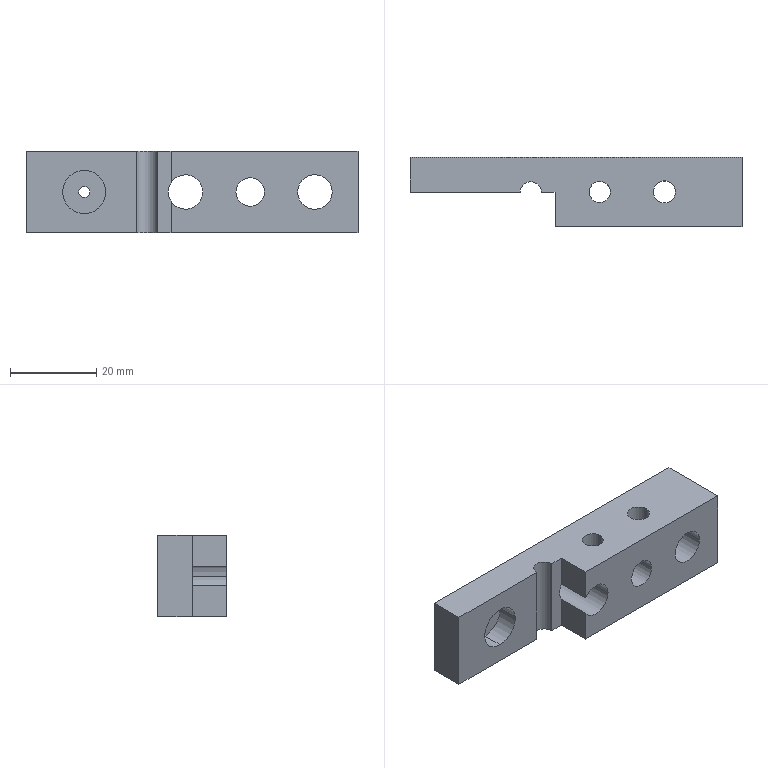Part | SolidWorks | features ICE 2, Extrusion 1 | 1 solid | 26 faces | box 77 x 16 x 19 mm | volume 14859 mm3 | cylinder 15 | plane 11 | commonest cylinder face diameters 8 x4 4.917 x3 2.599 x2 5.153 x2 6.647 x2 10 x2
STEP:
#1=CARTESIAN_POINT('',(13.5,5.,14.5));
#2=VERTEX_POINT('',#1);
#3=CARTESIAN_POINT('',(13.5,5.,4.5));
#4=VERTEX_POINT('',#3);
#5=CARTESIAN_POINT('',(13.5,5.,9.5));
#6=DIRECTION('',(0.,-1.,0.));
#7=DIRECTION('',(0.,0.,-1.));
#8=AXIS2_PLACEMENT_3D('',#5,#6,#7);
#9=CIRCLE('',#8,5.);
#10=EDGE_CURVE('',#2,#4,#9,.T.);
#11=ORIENTED_EDGE('',*,*,#10,.F.);
#12=CARTESIAN_POINT('',(13.5,0.,14.5));
#13=VERTEX_POINT('',#12);
#14=CARTESIAN_POINT('',(13.5,5.,14.5));
#15=DIRECTION('',(0.,-1.,0.));
#16=VECTOR('',#15,1000.);
#17=LINE('',#14,#16);
#18=EDGE_CURVE('',#2,#13,#17,.T.);
#19=ORIENTED_EDGE('',*,*,#18,.T.);
#20=CARTESIAN_POINT('',(13.5,0.,4.5));
#21=VERTEX_POINT('',#20);
#22=CARTESIAN_POINT('',(13.5,0.,9.5));
#23=DIRECTION('',(0.,-1.,0.));
#24=DIRECTION('',(0.,0.,-1.));
#25=AXIS2_PLACEMENT_3D('',#22,#23,#24);
#26=CIRCLE('',#25,5.);
#27=EDGE_CURVE('',#13,#21,#26,.T.);
#28=ORIENTED_EDGE('',*,*,#27,.T.);
#29=CARTESIAN_POINT('',(13.5,5.,4.5));
#30=DIRECTION('',(0.,-1.,0.));
#31=VECTOR('',#30,1000.);
#32=LINE('',#29,#31);
#33=EDGE_CURVE('',#4,#21,#32,.T.);
#34=ORIENTED_EDGE('',*,*,#33,.F.);
#35=EDGE_LOOP('',(#11,#19,#28,#34));
#36=FACE_OUTER_BOUND('',#35,.T.);
#37=CARTESIAN_POINT('',(13.5,5.,9.5));
#38=DIRECTION('',(0.,-1.,0.));
#39=DIRECTION('',(0.,0.,-1.));
#40=AXIS2_PLACEMENT_3D('',#37,#38,#39);
#41=CYLINDRICAL_SURFACE('',#40,5.);
#42=ADVANCED_FACE('',(#36),#41,.F.);
#43=CARTESIAN_POINT('',(71.,-7.907,9.5));
#44=VERTEX_POINT('',#43);
#45=CARTESIAN_POINT('',(63.,-7.907,9.5));
#46=VERTEX_POINT('',#45);
#47=CARTESIAN_POINT('',(67.,-7.907,9.5));
#48=DIRECTION('',(0.,1.,0.));
#49=DIRECTION('',(-1.,0.,0.));
#50=AXIS2_PLACEMENT_3D('',#47,#48,#49);
#51=CIRCLE('',#50,4.);
#52=EDGE_CURVE('',#44,#46,#51,.T.);
#53=ORIENTED_EDGE('',*,*,#52,.F.);
#54=CARTESIAN_POINT('',(71.,8.093,9.5));
#55=VERTEX_POINT('',#54);
#56=CARTESIAN_POINT('',(71.,-7.907,9.5));
#57=DIRECTION('',(0.,1.,0.));
#58=VECTOR('',#57,1000.);
#59=LINE('',#56,#58);
#60=EDGE_CURVE('',#44,#55,#59,.T.);
#61=ORIENTED_EDGE('',*,*,#60,.T.);
#62=CARTESIAN_POINT('',(63.,8.093,9.5));
#63=VERTEX_POINT('',#62);
#64=CARTESIAN_POINT('',(67.,8.093,9.5));
#65=DIRECTION('',(0.,1.,0.));
#66=DIRECTION('',(-1.,0.,0.));
#67=AXIS2_PLACEMENT_3D('',#64,#65,#66);
#68=CIRCLE('',#67,4.);
#69=EDGE_CURVE('',#55,#63,#68,.T.);
#70=ORIENTED_EDGE('',*,*,#69,.T.);
#71=CARTESIAN_POINT('',(63.,-7.907,9.5));
#72=DIRECTION('',(0.,1.,0.));
#73=VECTOR('',#72,1000.);
#74=LINE('',#71,#73);
#75=EDGE_CURVE('',#46,#63,#74,.T.);
#76=ORIENTED_EDGE('',*,*,#75,.F.);
#77=EDGE_LOOP('',(#53,#61,#70,#76));
#78=FACE_OUTER_BOUND('',#77,.T.);
#79=CARTESIAN_POINT('',(67.,-7.907,9.5));
#80=DIRECTION('',(0.,1.,0.));
#81=DIRECTION('',(-1.,0.,0.));
#82=AXIS2_PLACEMENT_3D('',#79,#80,#81);
#83=CYLINDRICAL_SURFACE('',#82,4.);
#84=ADVANCED_FACE('',(#78),#83,.F.);
#85=CARTESIAN_POINT('',(55.324,-7.907,9.5));
#86=VERTEX_POINT('',#85);
#87=CARTESIAN_POINT('',(48.677,-7.907,9.5));
#88=VERTEX_POINT('',#87);
#89=CARTESIAN_POINT('',(52.,-7.907,9.5));
#90=DIRECTION('',(0.,1.,0.));
#91=DIRECTION('',(-1.,0.,0.));
#92=AXIS2_PLACEMENT_3D('',#89,#90,#91);
#93=CIRCLE('',#92,3.324);
#94=EDGE_CURVE('',#86,#88,#93,.T.);
#95=ORIENTED_EDGE('',*,*,#94,.F.);
#96=CARTESIAN_POINT('',(55.324,8.093,9.5));
#97=VERTEX_POINT('',#96);
#98=CARTESIAN_POINT('',(55.324,-7.907,9.5));
#99=DIRECTION('',(0.,1.,0.));
#100=VECTOR('',#99,1000.);
#101=LINE('',#98,#100);
#102=EDGE_CURVE('',#86,#97,#101,.T.);
#103=ORIENTED_EDGE('',*,*,#102,.T.);
#104=CARTESIAN_POINT('',(48.677,8.093,9.5));
#105=VERTEX_POINT('',#104);
#106=CARTESIAN_POINT('',(52.,8.093,9.5));
#107=DIRECTION('',(0.,1.,0.));
#108=DIRECTION('',(-1.,0.,0.));
#109=AXIS2_PLACEMENT_3D('',#106,#107,#108);
#110=CIRCLE('',#109,3.324);
#111=EDGE_CURVE('',#97,#105,#110,.T.);
#112=ORIENTED_EDGE('',*,*,#111,.T.);
#113=CARTESIAN_POINT('',(48.677,-7.907,9.5));
#114=DIRECTION('',(0.,1.,0.));
#115=VECTOR('',#114,1000.);
#116=LINE('',#113,#115);
#117=EDGE_CURVE('',#88,#105,#116,.T.);
#118=ORIENTED_EDGE('',*,*,#117,.F.);
#119=EDGE_LOOP('',(#95,#103,#112,#118));
#120=FACE_OUTER_BOUND('',#119,.T.);
#121=CARTESIAN_POINT('',(52.,-7.907,9.5));
#122=DIRECTION('',(0.,1.,0.));
#123=DIRECTION('',(-1.,0.,0.));
#124=AXIS2_PLACEMENT_3D('',#121,#122,#123);
#125=CYLINDRICAL_SURFACE('',#124,3.324);
#126=ADVANCED_FACE('',(#120),#125,.F.);
#127=CARTESIAN_POINT('',(41.,-7.907,9.5));
#128=VERTEX_POINT('',#127);
#129=CARTESIAN_POINT('',(33.637,-7.907,7.334));
#130=VERTEX_POINT('',#129);
#131=CARTESIAN_POINT('',(37.,-7.907,9.5));
#132=DIRECTION('',(0.,1.,0.));
#133=DIRECTION('',(-1.,0.,0.));
#134=AXIS2_PLACEMENT_3D('',#131,#132,#133);
#135=CIRCLE('',#134,4.);
#136=EDGE_CURVE('',#128,#130,#135,.T.);
#137=ORIENTED_EDGE('',*,*,#136,.F.);
#138=CARTESIAN_POINT('',(41.,8.093,9.5));
#139=VERTEX_POINT('',#138);
#140=CARTESIAN_POINT('',(41.,-7.907,9.5));
#141=DIRECTION('',(0.,1.,0.));
#142=VECTOR('',#141,1000.);
#143=LINE('',#140,#142);
#144=EDGE_CURVE('',#128,#139,#143,.T.);
#145=ORIENTED_EDGE('',*,*,#144,.T.);
#146=CARTESIAN_POINT('',(33.,8.093,9.5));
#147=VERTEX_POINT('',#146);
#148=CARTESIAN_POINT('',(37.,8.093,9.5));
#149=DIRECTION('',(0.,1.,0.));
#150=DIRECTION('',(-1.,0.,0.));
#151=AXIS2_PLACEMENT_3D('',#148,#149,#150);
#152=CIRCLE('',#151,4.);
#153=EDGE_CURVE('',#139,#147,#152,.T.);
#154=ORIENTED_EDGE('',*,*,#153,.T.);
#155=CARTESIAN_POINT('',(33.,0.,9.5));
#156=VERTEX_POINT('',#155);
#157=CARTESIAN_POINT('',(33.,-7.907,9.5));
#158=DIRECTION('',(0.,1.,0.));
#159=VECTOR('',#158,1000.);
#160=LINE('',#157,#159);
#161=EDGE_CURVE('',#156,#147,#160,.T.);
#162=ORIENTED_EDGE('',*,*,#161,.F.);
#163=CARTESIAN_POINT('',(33.637,0.,7.334));
#164=VERTEX_POINT('',#163);
#165=CARTESIAN_POINT('',(37.,0.,9.5));
#166=DIRECTION('',(0.,1.,0.));
#167=DIRECTION('',(0.,0.,1.));
#168=AXIS2_PLACEMENT_3D('',#165,#166,#167);
#169=CIRCLE('',#168,4.);
#170=EDGE_CURVE('',#164,#156,#169,.T.);
#171=ORIENTED_EDGE('',*,*,#170,.F.);
#172=CARTESIAN_POINT('',(33.637,-7.907,7.334));
#173=DIRECTION('',(0.,1.,0.));
#174=VECTOR('',#173,1000.);
#175=LINE('',#172,#174);
#176=EDGE_CURVE('',#130,#164,#175,.T.);
#177=ORIENTED_EDGE('',*,*,#176,.F.);
#178=EDGE_LOOP('',(#137,#145,#154,#162,#171,#177));
#179=FACE_OUTER_BOUND('',#178,.T.);
#180=CARTESIAN_POINT('',(37.,-7.907,9.5));
#181=DIRECTION('',(0.,1.,0.));
#182=DIRECTION('',(-1.,0.,0.));
#183=AXIS2_PLACEMENT_3D('',#180,#181,#182);
#184=CYLINDRICAL_SURFACE('',#183,4.);
#185=ADVANCED_FACE('',(#179),#184,.F.);
#186=CARTESIAN_POINT('',(41.541,0.09258,19.));
#187=VERTEX_POINT('',#186);
#188=CARTESIAN_POINT('',(46.459,0.09258,19.));
#189=VERTEX_POINT('',#188);
#190=CARTESIAN_POINT('',(44.,0.09258,19.));
#191=DIRECTION('',(0.,0.,1.));
#192=DIRECTION('',(1.,0.,0.));
#193=AXIS2_PLACEMENT_3D('',#190,#191,#192);
#194=CIRCLE('',#193,2.459);
#195=EDGE_CURVE('',#187,#189,#194,.T.);
#196=ORIENTED_EDGE('',*,*,#195,.T.);
#197=CARTESIAN_POINT('',(46.459,0.09258,0.));
#198=VERTEX_POINT('',#197);
#199=CARTESIAN_POINT('',(46.459,0.09258,19.));
#200=DIRECTION('',(0.,0.,-1.));
#201=VECTOR('',#200,1000.);
#202=LINE('',#199,#201);
#203=EDGE_CURVE('',#189,#198,#202,.T.);
#204=ORIENTED_EDGE('',*,*,#203,.T.);
#205=CARTESIAN_POINT('',(41.541,0.09258,0.));
#206=VERTEX_POINT('',#205);
#207=CARTESIAN_POINT('',(44.,0.09258,0.));
#208=DIRECTION('',(0.,0.,1.));
#209=DIRECTION('',(1.,0.,0.));
#210=AXIS2_PLACEMENT_3D('',#207,#208,#209);
#211=CIRCLE('',#210,2.459);
#212=EDGE_CURVE('',#206,#198,#211,.T.);
#213=ORIENTED_EDGE('',*,*,#212,.F.);
#214=CARTESIAN_POINT('',(41.541,0.09258,19.));
#215=DIRECTION('',(0.,0.,-1.));
#216=VECTOR('',#215,1000.);
#217=LINE('',#214,#216);
#218=EDGE_CURVE('',#187,#206,#217,.T.);
#219=ORIENTED_EDGE('',*,*,#218,.F.);
#220=EDGE_LOOP('',(#196,#204,#213,#219));
#221=FACE_OUTER_BOUND('',#220,.T.);
#222=CARTESIAN_POINT('',(44.,0.09258,19.));
#223=DIRECTION('',(0.,0.,-1.));
#224=DIRECTION('',(-1.,0.,0.));
#225=AXIS2_PLACEMENT_3D('',#222,#223,#224);
#226=CYLINDRICAL_SURFACE('',#225,2.459);
#227=ADVANCED_FACE('',(#221),#226,.F.);
#228=CARTESIAN_POINT('',(56.424,0.09258,19.));
#229=VERTEX_POINT('',#228);
#230=CARTESIAN_POINT('',(61.576,0.09258,19.));
#231=VERTEX_POINT('',#230);
#232=CARTESIAN_POINT('',(59.,0.09258,19.));
#233=DIRECTION('',(0.,0.,1.));
#234=DIRECTION('',(1.,0.,0.));
#235=AXIS2_PLACEMENT_3D('',#232,#233,#234);
#236=CIRCLE('',#235,2.576);
#237=EDGE_CURVE('',#229,#231,#236,.T.);
#238=ORIENTED_EDGE('',*,*,#237,.T.);
#239=CARTESIAN_POINT('',(61.576,0.09258,0.));
#240=VERTEX_POINT('',#239);
#241=CARTESIAN_POINT('',(61.576,0.09258,19.));
#242=DIRECTION('',(0.,0.,-1.));
#243=VECTOR('',#242,1000.);
#244=LINE('',#241,#243);
#245=EDGE_CURVE('',#231,#240,#244,.T.);
#246=ORIENTED_EDGE('',*,*,#245,.T.);
#247=CARTESIAN_POINT('',(56.424,0.09258,0.));
#248=VERTEX_POINT('',#247);
#249=CARTESIAN_POINT('',(59.,0.09258,0.));
#250=DIRECTION('',(0.,0.,1.));
#251=DIRECTION('',(1.,0.,0.));
#252=AXIS2_PLACEMENT_3D('',#249,#250,#251);
#253=CIRCLE('',#252,2.576);
#254=EDGE_CURVE('',#248,#240,#253,.T.);
#255=ORIENTED_EDGE('',*,*,#254,.F.);
#256=CARTESIAN_POINT('',(56.424,0.09258,19.));
#257=DIRECTION('',(0.,0.,-1.));
#258=VECTOR('',#257,1000.);
#259=LINE('',#256,#258);
#260=EDGE_CURVE('',#229,#248,#259,.T.);
#261=ORIENTED_EDGE('',*,*,#260,.F.);
#262=EDGE_LOOP('',(#238,#246,#255,#261));
#263=FACE_OUTER_BOUND('',#262,.T.);
#264=CARTESIAN_POINT('',(59.,0.09258,19.));
#265=DIRECTION('',(0.,0.,-1.));
#266=DIRECTION('',(-1.,0.,0.));
#267=AXIS2_PLACEMENT_3D('',#264,#265,#266);
#268=CYLINDRICAL_SURFACE('',#267,2.576);
#269=ADVANCED_FACE('',(#263),#268,.F.);
#270=CARTESIAN_POINT('',(14.8,5.,9.5));
#271=VERTEX_POINT('',#270);
#272=CARTESIAN_POINT('',(12.201,5.,9.5));
#273=VERTEX_POINT('',#272);
#274=CARTESIAN_POINT('',(13.5,5.,9.5));
#275=DIRECTION('',(0.,1.,0.));
#276=DIRECTION('',(0.,0.,-1.));
#277=AXIS2_PLACEMENT_3D('',#274,#275,#276);
#278=CIRCLE('',#277,1.299);
#279=EDGE_CURVE('',#271,#273,#278,.T.);
#280=ORIENTED_EDGE('',*,*,#279,.F.);
#281=CARTESIAN_POINT('',(14.8,8.093,9.5));
#282=VERTEX_POINT('',#281);
#283=CARTESIAN_POINT('',(14.8,-7.907,9.5));
#284=DIRECTION('',(0.,1.,0.));
#285=VECTOR('',#284,1000.);
#286=LINE('',#283,#285);
#287=EDGE_CURVE('',#271,#282,#286,.T.);
#288=ORIENTED_EDGE('',*,*,#287,.T.);
#289=CARTESIAN_POINT('',(12.201,8.093,9.5));
#290=VERTEX_POINT('',#289);
#291=CARTESIAN_POINT('',(13.5,8.093,9.5));
#292=DIRECTION('',(0.,1.,0.));
#293=DIRECTION('',(-1.,0.,0.));
#294=AXIS2_PLACEMENT_3D('',#291,#292,#293);
#295=CIRCLE('',#294,1.299);
#296=EDGE_CURVE('',#282,#290,#295,.T.);
#297=ORIENTED_EDGE('',*,*,#296,.T.);
#298=CARTESIAN_POINT('',(12.201,-7.907,9.5));
#299=DIRECTION('',(0.,1.,0.));
#300=VECTOR('',#299,1000.);
#301=LINE('',#298,#300);
#302=EDGE_CURVE('',#273,#290,#301,.T.);
#303=ORIENTED_EDGE('',*,*,#302,.F.);
#304=EDGE_LOOP('',(#280,#288,#297,#303));
#305=FACE_OUTER_BOUND('',#304,.T.);
#306=CARTESIAN_POINT('',(13.5,-7.907,9.5));
#307=DIRECTION('',(0.,1.,0.));
#308=DIRECTION('',(-1.,0.,0.));
#309=AXIS2_PLACEMENT_3D('',#306,#307,#308);
#310=CYLINDRICAL_SURFACE('',#309,1.299);
#311=ADVANCED_FACE('',(#305),#310,.F.);
#312=ORIENTED_EDGE('',*,*,#287,.F.);
#313=CARTESIAN_POINT('',(13.5,5.,9.5));
#314=DIRECTION('',(0.,1.,0.));
#315=DIRECTION('',(0.,0.,-1.));
#316=AXIS2_PLACEMENT_3D('',#313,#314,#315);
#317=CIRCLE('',#316,1.299);
#318=EDGE_CURVE('',#273,#271,#317,.T.);
#319=ORIENTED_EDGE('',*,*,#318,.F.);
#320=ORIENTED_EDGE('',*,*,#302,.T.);
#321=CARTESIAN_POINT('',(13.5,8.093,9.5));
#322=DIRECTION('',(0.,1.,0.));
#323=DIRECTION('',(-1.,0.,0.));
#324=AXIS2_PLACEMENT_3D('',#321,#322,#323);
#325=CIRCLE('',#324,1.299);
#326=EDGE_CURVE('',#290,#282,#325,.T.);
#327=ORIENTED_EDGE('',*,*,#326,.T.);
#328=EDGE_LOOP('',(#312,#319,#320,#327));
#329=FACE_OUTER_BOUND('',#328,.T.);
#330=CARTESIAN_POINT('',(13.5,-7.907,9.5));
#331=DIRECTION('',(0.,1.,0.));
#332=DIRECTION('',(-1.,0.,0.));
#333=AXIS2_PLACEMENT_3D('',#330,#331,#332);
#334=CYLINDRICAL_SURFACE('',#333,1.299);
#335=ADVANCED_FACE('',(#329),#334,.F.);
#336=CARTESIAN_POINT('',(33.637,-7.907,0.));
#337=VERTEX_POINT('',#336);
#338=CARTESIAN_POINT('',(33.637,-7.907,19.));
#339=DIRECTION('',(0.,0.,-1.));
#340=VECTOR('',#339,1000.);
#341=LINE('',#338,#340);
#342=EDGE_CURVE('',#130,#337,#341,.T.);
#343=ORIENTED_EDGE('',*,*,#342,.F.);
#344=ORIENTED_EDGE('',*,*,#176,.T.);
#345=CARTESIAN_POINT('',(33.637,0.,0.));
#346=VERTEX_POINT('',#345);
#347=CARTESIAN_POINT('',(33.637,0.,19.));
#348=DIRECTION('',(0.,0.,-1.));
#349=VECTOR('',#348,1000.);
#350=LINE('',#347,#349);
#351=EDGE_CURVE('',#164,#346,#350,.T.);
#352=ORIENTED_EDGE('',*,*,#351,.T.);
#353=CARTESIAN_POINT('',(33.637,0.,0.));
#354=DIRECTION('',(0.,-1.,0.));
#355=VECTOR('',#354,1000.);
#356=LINE('',#353,#355);
#357=EDGE_CURVE('',#346,#337,#356,.T.);
#358=ORIENTED_EDGE('',*,*,#357,.T.);
#359=EDGE_LOOP('',(#343,#344,#352,#358));
#360=FACE_OUTER_BOUND('',#359,.T.);
#361=CARTESIAN_POINT('',(33.637,0.,19.));
#362=DIRECTION('',(1.,0.,0.));
#363=DIRECTION('',(0.,0.,-1.));
#364=AXIS2_PLACEMENT_3D('',#361,#362,#363);
#365=PLANE('',#364);
#366=ADVANCED_FACE('',(#360),#365,.F.);
#367=ORIENTED_EDGE('',*,*,#237,.F.);
#368=CARTESIAN_POINT('',(59.,0.09258,19.));
#369=DIRECTION('',(0.,0.,1.));
#370=DIRECTION('',(1.,0.,0.));
#371=AXIS2_PLACEMENT_3D('',#368,#369,#370);
#372=CIRCLE('',#371,2.576);
#373=EDGE_CURVE('',#231,#229,#372,.T.);
#374=ORIENTED_EDGE('',*,*,#373,.F.);
#375=EDGE_LOOP('',(#367,#374));
#376=FACE_BOUND('',#375,.T.);
#377=CARTESIAN_POINT('',(0.,8.093,19.));
#378=VERTEX_POINT('',#377);
#379=CARTESIAN_POINT('',(0.,0.,19.));
#380=VERTEX_POINT('',#379);
#381=CARTESIAN_POINT('',(0.,8.093,19.));
#382=DIRECTION('',(0.,-1.,0.));
#383=VECTOR('',#382,1000.);
#384=LINE('',#381,#383);
#385=EDGE_CURVE('',#378,#380,#384,.T.);
#386=ORIENTED_EDGE('',*,*,#385,.T.);
#387=CARTESIAN_POINT('',(25.541,0.,19.));
#388=VERTEX_POINT('',#387);
#389=CARTESIAN_POINT('',(0.,0.,19.));
#390=DIRECTION('',(1.,0.,0.));
#391=VECTOR('',#390,1000.);
#392=LINE('',#389,#391);
#393=EDGE_CURVE('',#380,#388,#392,.T.);
#394=ORIENTED_EDGE('',*,*,#393,.T.);
#395=CARTESIAN_POINT('',(30.458,0.,19.));
#396=VERTEX_POINT('',#395);
#397=CARTESIAN_POINT('',(28.,0.,19.));
#398=DIRECTION('',(0.,0.,-1.));
#399=DIRECTION('',(1.,0.,0.));
#400=AXIS2_PLACEMENT_3D('',#397,#398,#399);
#401=CIRCLE('',#400,2.458);
#402=EDGE_CURVE('',#388,#396,#401,.T.);
#403=ORIENTED_EDGE('',*,*,#402,.T.);
#404=CARTESIAN_POINT('',(33.637,0.,19.));
#405=VERTEX_POINT('',#404);
#406=CARTESIAN_POINT('',(30.458,0.,19.));
#407=DIRECTION('',(1.,0.,0.));
#408=VECTOR('',#407,1000.);
#409=LINE('',#406,#408);
#410=EDGE_CURVE('',#396,#405,#409,.T.);
#411=ORIENTED_EDGE('',*,*,#410,.T.);
#412=CARTESIAN_POINT('',(33.637,-7.907,19.));
#413=VERTEX_POINT('',#412);
#414=CARTESIAN_POINT('',(33.637,0.,19.));
#415=DIRECTION('',(0.,-1.,0.));
#416=VECTOR('',#415,1000.);
#417=LINE('',#414,#416);
#418=EDGE_CURVE('',#405,#413,#417,.T.);
#419=ORIENTED_EDGE('',*,*,#418,.T.);
#420=CARTESIAN_POINT('',(77.,-7.907,19.));
#421=VERTEX_POINT('',#420);
#422=CARTESIAN_POINT('',(33.637,-7.907,19.));
#423=DIRECTION('',(1.,0.,0.));
#424=VECTOR('',#423,1000.);
#425=LINE('',#422,#424);
#426=EDGE_CURVE('',#413,#421,#425,.T.);
#427=ORIENTED_EDGE('',*,*,#426,.T.);
#428=CARTESIAN_POINT('',(77.,8.093,19.));
#429=VERTEX_POINT('',#428);
#430=CARTESIAN_POINT('',(77.,-7.907,19.));
#431=DIRECTION('',(0.,1.,0.));
#432=VECTOR('',#431,1000.);
#433=LINE('',#430,#432);
#434=EDGE_CURVE('',#421,#429,#433,.T.);
#435=ORIENTED_EDGE('',*,*,#434,.T.);
#436=CARTESIAN_POINT('',(77.,8.093,19.));
#437=DIRECTION('',(-1.,0.,0.));
#438=VECTOR('',#437,1000.);
#439=LINE('',#436,#438);
#440=EDGE_CURVE('',#429,#378,#439,.T.);
#441=ORIENTED_EDGE('',*,*,#440,.T.);
#442=EDGE_LOOP('',(#386,#394,#403,#411,#419,#427,#435,#441));
#443=FACE_OUTER_BOUND('',#442,.T.);
#444=ORIENTED_EDGE('',*,*,#195,.F.);
#445=CARTESIAN_POINT('',(44.,0.09258,19.));
#446=DIRECTION('',(0.,0.,1.));
#447=DIRECTION('',(1.,0.,0.));
#448=AXIS2_PLACEMENT_3D('',#445,#446,#447);
#449=CIRCLE('',#448,2.459);
#450=EDGE_CURVE('',#189,#187,#449,.T.);
#451=ORIENTED_EDGE('',*,*,#450,.F.);
#452=EDGE_LOOP('',(#444,#451));
#453=FACE_BOUND('',#452,.T.);
#454=CARTESIAN_POINT('',(28.,0.,19.));
#455=DIRECTION('',(0.,0.,1.));
#456=DIRECTION('',(1.,0.,0.));
#457=AXIS2_PLACEMENT_3D('',#454,#455,#456);
#458=PLANE('',#457);
#459=ADVANCED_FACE('',(#376,#443,#453),#458,.T.);
#460=CARTESIAN_POINT('',(0.,8.093,0.));
#461=VERTEX_POINT('',#460);
#462=CARTESIAN_POINT('',(0.,0.,0.));
#463=VERTEX_POINT('',#462);
#464=CARTESIAN_POINT('',(0.,8.093,0.));
#465=DIRECTION('',(0.,-1.,0.));
#466=VECTOR('',#465,1000.);
#467=LINE('',#464,#466);
#468=EDGE_CURVE('',#461,#463,#467,.T.);
#469=ORIENTED_EDGE('',*,*,#468,.F.);
#470=CARTESIAN_POINT('',(77.,8.093,0.));
#471=VERTEX_POINT('',#470);
#472=CARTESIAN_POINT('',(77.,8.093,0.));
#473=DIRECTION('',(-1.,0.,0.));
#474=VECTOR('',#473,1000.);
#475=LINE('',#472,#474);
#476=EDGE_CURVE('',#471,#461,#475,.T.);
#477=ORIENTED_EDGE('',*,*,#476,.F.);
#478=CARTESIAN_POINT('',(77.,-7.907,0.));
#479=VERTEX_POINT('',#478);
#480=CARTESIAN_POINT('',(77.,-7.907,0.));
#481=DIRECTION('',(0.,1.,0.));
#482=VECTOR('',#481,1000.);
#483=LINE('',#480,#482);
#484=EDGE_CURVE('',#479,#471,#483,.T.);
#485=ORIENTED_EDGE('',*,*,#484,.F.);
#486=CARTESIAN_POINT('',(33.637,-7.907,0.));
#487=DIRECTION('',(1.,0.,0.));
#488=VECTOR('',#487,1000.);
#489=LINE('',#486,#488);
#490=EDGE_CURVE('',#337,#479,#489,.T.);
#491=ORIENTED_EDGE('',*,*,#490,.F.);
#492=ORIENTED_EDGE('',*,*,#357,.F.);
#493=CARTESIAN_POINT('',(30.458,0.,0.));
#494=VERTEX_POINT('',#493);
#495=CARTESIAN_POINT('',(30.458,0.,0.));
#496=DIRECTION('',(1.,0.,0.));
#497=VECTOR('',#496,1000.);
#498=LINE('',#495,#497);
#499=EDGE_CURVE('',#494,#346,#498,.T.);
#500=ORIENTED_EDGE('',*,*,#499,.F.);
#501=CARTESIAN_POINT('',(25.541,0.,0.));
#502=VERTEX_POINT('',#501);
#503=CARTESIAN_POINT('',(28.,0.,0.));
#504=DIRECTION('',(0.,0.,-1.));
#505=DIRECTION('',(1.,0.,0.));
#506=AXIS2_PLACEMENT_3D('',#503,#504,#505);
#507=CIRCLE('',#506,2.458);
#508=EDGE_CURVE('',#502,#494,#507,.T.);
#509=ORIENTED_EDGE('',*,*,#508,.F.);
#510=CARTESIAN_POINT('',(0.,0.,0.));
#511=DIRECTION('',(1.,0.,0.));
#512=VECTOR('',#511,1000.);
#513=LINE('',#510,#512);
#514=EDGE_CURVE('',#463,#502,#513,.T.);
#515=ORIENTED_EDGE('',*,*,#514,.F.);
#516=EDGE_LOOP('',(#469,#477,#485,#491,#492,#500,#509,#515));
#517=FACE_OUTER_BOUND('',#516,.T.);
#518=ORIENTED_EDGE('',*,*,#254,.T.);
#519=CARTESIAN_POINT('',(59.,0.09258,0.));
#520=DIRECTION('',(0.,0.,1.));
#521=DIRECTION('',(1.,0.,0.));
#522=AXIS2_PLACEMENT_3D('',#519,#520,#521);
#523=CIRCLE('',#522,2.576);
#524=EDGE_CURVE('',#240,#248,#523,.T.);
#525=ORIENTED_EDGE('',*,*,#524,.T.);
#526=EDGE_LOOP('',(#518,#525));
#527=FACE_BOUND('',#526,.T.);
#528=ORIENTED_EDGE('',*,*,#212,.T.);
#529=CARTESIAN_POINT('',(44.,0.09258,0.));
#530=DIRECTION('',(0.,0.,1.));
#531=DIRECTION('',(1.,0.,0.));
#532=AXIS2_PLACEMENT_3D('',#529,#530,#531);
#533=CIRCLE('',#532,2.459);
#534=EDGE_CURVE('',#198,#206,#533,.T.);
#535=ORIENTED_EDGE('',*,*,#534,.T.);
#536=EDGE_LOOP('',(#528,#535));
#537=FACE_BOUND('',#536,.T.);
#538=CARTESIAN_POINT('',(28.,0.,0.));
#539=DIRECTION('',(0.,0.,1.));
#540=DIRECTION('',(1.,0.,0.));
#541=AXIS2_PLACEMENT_3D('',#538,#539,#540);
#542=PLANE('',#541);
#543=ADVANCED_FACE('',(#517,#527,#537),#542,.F.);
#544=ORIENTED_EDGE('',*,*,#468,.T.);
#545=CARTESIAN_POINT('',(0.,0.,19.));
#546=DIRECTION('',(0.,0.,-1.));
#547=VECTOR('',#546,1000.);
#548=LINE('',#545,#547);
#549=EDGE_CURVE('',#380,#463,#548,.T.);
#550=ORIENTED_EDGE('',*,*,#549,.F.);
#551=ORIENTED_EDGE('',*,*,#385,.F.);
#552=CARTESIAN_POINT('',(0.,8.093,19.));
#553=DIRECTION('',(0.,0.,-1.));
#554=VECTOR('',#553,1000.);
#555=LINE('',#552,#554);
#556=EDGE_CURVE('',#378,#461,#555,.T.);
#557=ORIENTED_EDGE('',*,*,#556,.T.);
#558=EDGE_LOOP('',(#544,#550,#551,#557));
#559=FACE_OUTER_BOUND('',#558,.T.);
#560=CARTESIAN_POINT('',(0.,8.093,19.));
#561=DIRECTION('',(1.,0.,0.));
#562=DIRECTION('',(0.,1.,0.));
#563=AXIS2_PLACEMENT_3D('',#560,#561,#562);
#564=PLANE('',#563);
#565=ADVANCED_FACE('',(#559),#564,.F.);
#566=CARTESIAN_POINT('',(13.5,0.,9.5));
#567=DIRECTION('',(0.,-1.,0.));
#568=DIRECTION('',(0.,0.,-1.));
#569=AXIS2_PLACEMENT_3D('',#566,#567,#568);
#570=CIRCLE('',#569,5.);
#571=EDGE_CURVE('',#21,#13,#570,.T.);
#572=ORIENTED_EDGE('',*,*,#571,.F.);
#573=ORIENTED_EDGE('',*,*,#27,.F.);
#574=EDGE_LOOP('',(#572,#573));
#575=FACE_BOUND('',#574,.T.);
#576=ORIENTED_EDGE('',*,*,#514,.T.);
#577=CARTESIAN_POINT('',(25.541,0.,19.));
#578=DIRECTION('',(0.,0.,-1.));
#579=VECTOR('',#578,1000.);
#580=LINE('',#577,#579);
#581=EDGE_CURVE('',#388,#502,#580,.T.);
#582=ORIENTED_EDGE('',*,*,#581,.F.);
#583=ORIENTED_EDGE('',*,*,#393,.F.);
#584=ORIENTED_EDGE('',*,*,#549,.T.);
#585=EDGE_LOOP('',(#576,#582,#583,#584));
#586=FACE_OUTER_BOUND('',#585,.T.);
#587=CARTESIAN_POINT('',(0.,0.,19.));
#588=DIRECTION('',(0.,1.,0.));
#589=DIRECTION('',(0.,0.,1.));
#590=AXIS2_PLACEMENT_3D('',#587,#588,#589);
#591=PLANE('',#590);
#592=ADVANCED_FACE('',(#575,#586),#591,.F.);
#593=ORIENTED_EDGE('',*,*,#508,.T.);
#594=CARTESIAN_POINT('',(30.458,0.,19.));
#595=DIRECTION('',(0.,0.,-1.));
#596=VECTOR('',#595,1000.);
#597=LINE('',#594,#596);
#598=EDGE_CURVE('',#396,#494,#597,.T.);
#599=ORIENTED_EDGE('',*,*,#598,.F.);
#600=ORIENTED_EDGE('',*,*,#402,.F.);
#601=ORIENTED_EDGE('',*,*,#581,.T.);
#602=EDGE_LOOP('',(#593,#599,#600,#601));
#603=FACE_OUTER_BOUND('',#602,.T.);
#604=CARTESIAN_POINT('',(28.,0.,19.));
#605=DIRECTION('',(0.,0.,-1.));
#606=DIRECTION('',(-1.,0.,0.));
#607=AXIS2_PLACEMENT_3D('',#604,#605,#606);
#608=CYLINDRICAL_SURFACE('',#607,2.458);
#609=ADVANCED_FACE('',(#603),#608,.F.);
#610=ORIENTED_EDGE('',*,*,#351,.F.);
#611=ORIENTED_EDGE('',*,*,#170,.T.);
#612=CARTESIAN_POINT('',(33.637,0.,11.666));
#613=VERTEX_POINT('',#612);
#614=CARTESIAN_POINT('',(37.,0.,9.5));
#615=DIRECTION('',(0.,1.,0.));
#616=DIRECTION('',(0.,0.,1.));
#617=AXIS2_PLACEMENT_3D('',#614,#615,#616);
#618=CIRCLE('',#617,4.);
#619=EDGE_CURVE('',#156,#613,#618,.T.);
#620=ORIENTED_EDGE('',*,*,#619,.T.);
#621=CARTESIAN_POINT('',(33.637,0.,19.));
#622=DIRECTION('',(0.,0.,-1.));
#623=VECTOR('',#622,1000.);
#624=LINE('',#621,#623);
#625=EDGE_CURVE('',#405,#613,#624,.T.);
#626=ORIENTED_EDGE('',*,*,#625,.F.);
#627=ORIENTED_EDGE('',*,*,#410,.F.);
#628=ORIENTED_EDGE('',*,*,#598,.T.);
#629=ORIENTED_EDGE('',*,*,#499,.T.);
#630=EDGE_LOOP('',(#610,#611,#620,#626,#627,#628,#629));
#631=FACE_OUTER_BOUND('',#630,.T.);
#632=CARTESIAN_POINT('',(30.458,0.,19.));
#633=DIRECTION('',(0.,1.,0.));
#634=DIRECTION('',(0.,0.,1.));
#635=AXIS2_PLACEMENT_3D('',#632,#633,#634);
#636=PLANE('',#635);
#637=ADVANCED_FACE('',(#631),#636,.F.);
#638=ORIENTED_EDGE('',*,*,#625,.T.);
#639=CARTESIAN_POINT('',(33.637,-7.907,11.666));
#640=VERTEX_POINT('',#639);
#641=CARTESIAN_POINT('',(33.637,-7.907,11.666));
#642=DIRECTION('',(0.,-1.,0.));
#643=VECTOR('',#642,1000.);
#644=LINE('',#641,#643);
#645=EDGE_CURVE('',#613,#640,#644,.T.);
#646=ORIENTED_EDGE('',*,*,#645,.T.);
#647=CARTESIAN_POINT('',(33.637,-7.907,19.));
#648=DIRECTION('',(0.,0.,-1.));
#649=VECTOR('',#648,1000.);
#650=LINE('',#647,#649);
#651=EDGE_CURVE('',#413,#640,#650,.T.);
#652=ORIENTED_EDGE('',*,*,#651,.F.);
#653=ORIENTED_EDGE('',*,*,#418,.F.);
#654=EDGE_LOOP('',(#638,#646,#652,#653));
#655=FACE_OUTER_BOUND('',#654,.T.);
#656=CARTESIAN_POINT('',(33.637,0.,19.));
#657=DIRECTION('',(1.,0.,0.));
#658=DIRECTION('',(0.,0.,-1.));
#659=AXIS2_PLACEMENT_3D('',#656,#657,#658);
#660=PLANE('',#659);
#661=ADVANCED_FACE('',(#655),#660,.F.);
#662=CARTESIAN_POINT('',(67.,-7.907,9.5));
#663=DIRECTION('',(0.,1.,0.));
#664=DIRECTION('',(-1.,0.,0.));
#665=AXIS2_PLACEMENT_3D('',#662,#663,#664);
#666=CIRCLE('',#665,4.);
#667=EDGE_CURVE('',#46,#44,#666,.T.);
#668=ORIENTED_EDGE('',*,*,#667,.T.);
#669=ORIENTED_EDGE('',*,*,#52,.T.);
#670=EDGE_LOOP('',(#668,#669));
#671=FACE_BOUND('',#670,.T.);
#672=CARTESIAN_POINT('',(52.,-7.907,9.5));
#673=DIRECTION('',(0.,1.,0.));
#674=DIRECTION('',(-1.,0.,0.));
#675=AXIS2_PLACEMENT_3D('',#672,#673,#674);
#676=CIRCLE('',#675,3.324);
#677=EDGE_CURVE('',#88,#86,#676,.T.);
#678=ORIENTED_EDGE('',*,*,#677,.T.);
#679=ORIENTED_EDGE('',*,*,#94,.T.);
#680=EDGE_LOOP('',(#678,#679));
#681=FACE_BOUND('',#680,.T.);
#682=ORIENTED_EDGE('',*,*,#651,.T.);
#683=CARTESIAN_POINT('',(37.,-7.907,9.5));
#684=DIRECTION('',(0.,1.,0.));
#685=DIRECTION('',(-1.,0.,0.));
#686=AXIS2_PLACEMENT_3D('',#683,#684,#685);
#687=CIRCLE('',#686,4.);
#688=EDGE_CURVE('',#640,#128,#687,.T.);
#689=ORIENTED_EDGE('',*,*,#688,.T.);
#690=ORIENTED_EDGE('',*,*,#136,.T.);
#691=ORIENTED_EDGE('',*,*,#342,.T.);
#692=ORIENTED_EDGE('',*,*,#490,.T.);
#693=CARTESIAN_POINT('',(77.,-7.907,19.));
#694=DIRECTION('',(0.,0.,-1.));
#695=VECTOR('',#694,1000.);
#696=LINE('',#693,#695);
#697=EDGE_CURVE('',#421,#479,#696,.T.);
#698=ORIENTED_EDGE('',*,*,#697,.F.);
#699=ORIENTED_EDGE('',*,*,#426,.F.);
#700=EDGE_LOOP('',(#682,#689,#690,#691,#692,#698,#699));
#701=FACE_OUTER_BOUND('',#700,.T.);
#702=CARTESIAN_POINT('',(33.637,-7.907,19.));
#703=DIRECTION('',(0.,1.,0.));
#704=DIRECTION('',(0.,0.,1.));
#705=AXIS2_PLACEMENT_3D('',#702,#703,#704);
#706=PLANE('',#705);
#707=ADVANCED_FACE('',(#671,#681,#701),#706,.F.);
#708=ORIENTED_EDGE('',*,*,#484,.T.);
#709=CARTESIAN_POINT('',(77.,8.093,19.));
#710=DIRECTION('',(0.,0.,-1.));
#711=VECTOR('',#710,1000.);
#712=LINE('',#709,#711);
#713=EDGE_CURVE('',#429,#471,#712,.T.);
#714=ORIENTED_EDGE('',*,*,#713,.F.);
#715=ORIENTED_EDGE('',*,*,#434,.F.);
#716=ORIENTED_EDGE('',*,*,#697,.T.);
#717=EDGE_LOOP('',(#708,#714,#715,#716));
#718=FACE_OUTER_BOUND('',#717,.T.);
#719=CARTESIAN_POINT('',(77.,-7.907,19.));
#720=DIRECTION('',(-1.,0.,0.));
#721=DIRECTION('',(0.,0.,1.));
#722=AXIS2_PLACEMENT_3D('',#719,#720,#721);
#723=PLANE('',#722);
#724=ADVANCED_FACE('',(#718),#723,.F.);
#725=CARTESIAN_POINT('',(67.,8.093,9.5));
#726=DIRECTION('',(0.,1.,0.));
#727=DIRECTION('',(-1.,0.,0.));
#728=AXIS2_PLACEMENT_3D('',#725,#726,#727);
#729=CIRCLE('',#728,4.);
#730=EDGE_CURVE('',#63,#55,#729,.T.);
#731=ORIENTED_EDGE('',*,*,#730,.F.);
#732=ORIENTED_EDGE('',*,*,#69,.F.);
#733=EDGE_LOOP('',(#731,#732));
#734=FACE_BOUND('',#733,.T.);
#735=CARTESIAN_POINT('',(52.,8.093,9.5));
#736=DIRECTION('',(0.,1.,0.));
#737=DIRECTION('',(-1.,0.,0.));
#738=AXIS2_PLACEMENT_3D('',#735,#736,#737);
#739=CIRCLE('',#738,3.324);
#740=EDGE_CURVE('',#105,#97,#739,.T.);
#741=ORIENTED_EDGE('',*,*,#740,.F.);
#742=ORIENTED_EDGE('',*,*,#111,.F.);
#743=EDGE_LOOP('',(#741,#742));
#744=FACE_BOUND('',#743,.T.);
#745=CARTESIAN_POINT('',(37.,8.093,9.5));
#746=DIRECTION('',(0.,1.,0.));
#747=DIRECTION('',(-1.,0.,0.));
#748=AXIS2_PLACEMENT_3D('',#745,#746,#747);
#749=CIRCLE('',#748,4.);
#750=EDGE_CURVE('',#147,#139,#749,.T.);
#751=ORIENTED_EDGE('',*,*,#750,.F.);
#752=ORIENTED_EDGE('',*,*,#153,.F.);
#753=EDGE_LOOP('',(#751,#752));
#754=FACE_BOUND('',#753,.T.);
#755=ORIENTED_EDGE('',*,*,#326,.F.);
#756=ORIENTED_EDGE('',*,*,#296,.F.);
#757=EDGE_LOOP('',(#755,#756));
#758=FACE_BOUND('',#757,.T.);
#759=ORIENTED_EDGE('',*,*,#476,.T.);
#760=ORIENTED_EDGE('',*,*,#556,.F.);
#761=ORIENTED_EDGE('',*,*,#440,.F.);
#762=ORIENTED_EDGE('',*,*,#713,.T.);
#763=EDGE_LOOP('',(#759,#760,#761,#762));
#764=FACE_OUTER_BOUND('',#763,.T.);
#765=CARTESIAN_POINT('',(77.,8.093,19.));
#766=DIRECTION('',(0.,-1.,0.));
#767=DIRECTION('',(1.,0.,0.));
#768=AXIS2_PLACEMENT_3D('',#765,#766,#767);
#769=PLANE('',#768);
#770=ADVANCED_FACE('',(#734,#744,#754,#758,#764),#769,.F.);
#771=ORIENTED_EDGE('',*,*,#245,.F.);
#772=ORIENTED_EDGE('',*,*,#373,.T.);
#773=ORIENTED_EDGE('',*,*,#260,.T.);
#774=ORIENTED_EDGE('',*,*,#524,.F.);
#775=EDGE_LOOP('',(#771,#772,#773,#774));
#776=FACE_OUTER_BOUND('',#775,.T.);
#777=CARTESIAN_POINT('',(59.,0.09258,19.));
#778=DIRECTION('',(0.,0.,-1.));
#779=DIRECTION('',(-1.,0.,0.));
#780=AXIS2_PLACEMENT_3D('',#777,#778,#779);
#781=CYLINDRICAL_SURFACE('',#780,2.576);
#782=ADVANCED_FACE('',(#776),#781,.F.);
#783=ORIENTED_EDGE('',*,*,#203,.F.);
#784=ORIENTED_EDGE('',*,*,#450,.T.);
#785=ORIENTED_EDGE('',*,*,#218,.T.);
#786=ORIENTED_EDGE('',*,*,#534,.F.);
#787=EDGE_LOOP('',(#783,#784,#785,#786));
#788=FACE_OUTER_BOUND('',#787,.T.);
#789=CARTESIAN_POINT('',(44.,0.09258,19.));
#790=DIRECTION('',(0.,0.,-1.));
#791=DIRECTION('',(-1.,0.,0.));
#792=AXIS2_PLACEMENT_3D('',#789,#790,#791);
#793=CYLINDRICAL_SURFACE('',#792,2.459);
#794=ADVANCED_FACE('',(#788),#793,.F.);
#795=ORIENTED_EDGE('',*,*,#144,.F.);
#796=ORIENTED_EDGE('',*,*,#688,.F.);
#797=ORIENTED_EDGE('',*,*,#645,.F.);
#798=ORIENTED_EDGE('',*,*,#619,.F.);
#799=ORIENTED_EDGE('',*,*,#161,.T.);
#800=ORIENTED_EDGE('',*,*,#750,.T.);
#801=EDGE_LOOP('',(#795,#796,#797,#798,#799,#800));
#802=FACE_OUTER_BOUND('',#801,.T.);
#803=CARTESIAN_POINT('',(37.,-7.907,9.5));
#804=DIRECTION('',(0.,1.,0.));
#805=DIRECTION('',(-1.,0.,0.));
#806=AXIS2_PLACEMENT_3D('',#803,#804,#805);
#807=CYLINDRICAL_SURFACE('',#806,4.);
#808=ADVANCED_FACE('',(#802),#807,.F.);
#809=ORIENTED_EDGE('',*,*,#102,.F.);
#810=ORIENTED_EDGE('',*,*,#677,.F.);
#811=ORIENTED_EDGE('',*,*,#117,.T.);
#812=ORIENTED_EDGE('',*,*,#740,.T.);
#813=EDGE_LOOP('',(#809,#810,#811,#812));
#814=FACE_OUTER_BOUND('',#813,.T.);
#815=CARTESIAN_POINT('',(52.,-7.907,9.5));
#816=DIRECTION('',(0.,1.,0.));
#817=DIRECTION('',(-1.,0.,0.));
#818=AXIS2_PLACEMENT_3D('',#815,#816,#817);
#819=CYLINDRICAL_SURFACE('',#818,3.324);
#820=ADVANCED_FACE('',(#814),#819,.F.);
#821=ORIENTED_EDGE('',*,*,#60,.F.);
#822=ORIENTED_EDGE('',*,*,#667,.F.);
#823=ORIENTED_EDGE('',*,*,#75,.T.);
#824=ORIENTED_EDGE('',*,*,#730,.T.);
#825=EDGE_LOOP('',(#821,#822,#823,#824));
#826=FACE_OUTER_BOUND('',#825,.T.);
#827=CARTESIAN_POINT('',(67.,-7.907,9.5));
#828=DIRECTION('',(0.,1.,0.));
#829=DIRECTION('',(-1.,0.,0.));
#830=AXIS2_PLACEMENT_3D('',#827,#828,#829);
#831=CYLINDRICAL_SURFACE('',#830,4.);
#832=ADVANCED_FACE('',(#826),#831,.F.);
#833=CARTESIAN_POINT('',(13.5,5.,9.5));
#834=DIRECTION('',(0.,-1.,0.));
#835=DIRECTION('',(0.,0.,-1.));
#836=AXIS2_PLACEMENT_3D('',#833,#834,#835);
#837=CIRCLE('',#836,5.);
#838=EDGE_CURVE('',#4,#2,#837,.T.);
#839=ORIENTED_EDGE('',*,*,#838,.T.);
#840=ORIENTED_EDGE('',*,*,#10,.T.);
#841=EDGE_LOOP('',(#839,#840));
#842=FACE_OUTER_BOUND('',#841,.T.);
#843=ORIENTED_EDGE('',*,*,#318,.T.);
#844=ORIENTED_EDGE('',*,*,#279,.T.);
#845=EDGE_LOOP('',(#843,#844));
#846=FACE_BOUND('',#845,.T.);
#847=CARTESIAN_POINT('',(13.5,5.,9.5));
#848=DIRECTION('',(0.,-1.,0.));
#849=DIRECTION('',(0.,0.,-1.));
#850=AXIS2_PLACEMENT_3D('',#847,#848,#849);
#851=PLANE('',#850);
#852=ADVANCED_FACE('',(#842,#846),#851,.T.);
#853=ORIENTED_EDGE('',*,*,#18,.F.);
#854=ORIENTED_EDGE('',*,*,#838,.F.);
#855=ORIENTED_EDGE('',*,*,#33,.T.);
#856=ORIENTED_EDGE('',*,*,#571,.T.);
#857=EDGE_LOOP('',(#853,#854,#855,#856));
#858=FACE_OUTER_BOUND('',#857,.T.);
#859=CARTESIAN_POINT('',(13.5,5.,9.5));
#860=DIRECTION('',(0.,-1.,0.));
#861=DIRECTION('',(0.,0.,-1.));
#862=AXIS2_PLACEMENT_3D('',#859,#860,#861);
#863=CYLINDRICAL_SURFACE('',#862,5.);
#864=ADVANCED_FACE('',(#858),#863,.F.);
#865=CLOSED_SHELL('',(#42,#84,#126,#185,#227,#269,#311,#335,#366,#459,#543,#565,#592,#609,#637,#661,#707,#724,#770,#782,#794,#808,#820,#832,#852,#864));
#866=MANIFOLD_SOLID_BREP('',#865);
#867=CARTESIAN_POINT('',(0.,0.,0.));
#868=DIRECTION('',(0.,0.,1.));
#869=DIRECTION('',(1.,0.,0.));
#870=AXIS2_PLACEMENT_3D('',#867,#868,#869);
#871=(LENGTH_UNIT()NAMED_UNIT(*)SI_UNIT(.MILLI.,.METRE.));
#872=UNCERTAINTY_MEASURE_WITH_UNIT(LENGTH_MEASURE(0.00001),#871,'','');
#873=(NAMED_UNIT(*)PLANE_ANGLE_UNIT()SI_UNIT($,.RADIAN.));
#874=(NAMED_UNIT(*)SI_UNIT($,.STERADIAN.)SOLID_ANGLE_UNIT());
#875=(GEOMETRIC_REPRESENTATION_CONTEXT(3)GLOBAL_UNCERTAINTY_ASSIGNED_CONTEXT((#872))GLOBAL_UNIT_ASSIGNED_CONTEXT((#871,#873,#874))REPRESENTATION_CONTEXT('',''));
#876=ADVANCED_BREP_SHAPE_REPRESENTATION('',(#866,#870),#875);